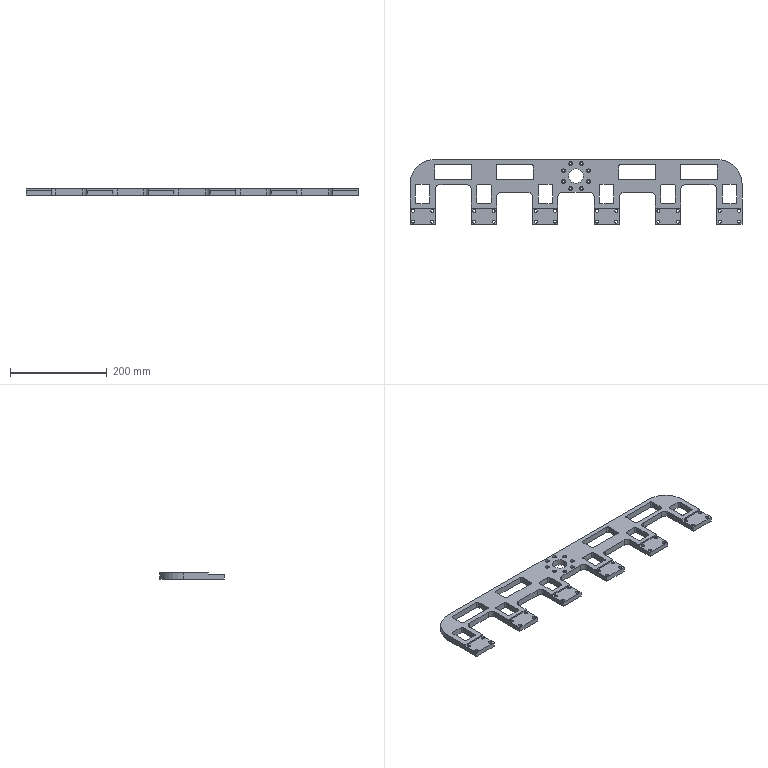NC program | NX | posted with a generic post | part box 687 x 134 x 13 mm
Lines 1 to 122 of 9954:
N10 G17 G21 G94 G90
(FLOOR_WALL_COPY , TOOL : D63)
N12 T01 M6
N14 G54
N16 G17 G0 G90 X-380. Y68.997 S6500 M3
N18 G43 Z30. H1
N20 Z3.
N22 G94 G1 Z0. F1500.
N24 X-377.
N26 X377.
N28 Y40.798
N30 X-377.
N32 Y12.599
N34 X377.
N36 Y-15.601
N38 X-377.
N40 Y-24.911
N42 Y-43.8
N44 X377.
N46 X380.
N48 Z3.
N50 G0 Z30.
N52 M5
(DRILLING_COPY_1 , TOOL : D6A45)
N54 T07 M6
N56 G54
N58 G17 G0 G90 X337.5 Y-39.2 S5000 M3
N60 G43 Z30. H7
N62 G94 G81 G98 Z-1. F250. R3.
N64 Y-61.2
N66 X297.5
N68 Y-39.2
N70 X210.5
N72 Y-61.2
N74 X170.5
N76 Y-39.2
N78 X83.5
N80 Y-61.2
N82 X43.5
N84 Y-39.2
N86 X10.715 Y7.131
N88 X25.869 Y22.285
N90 Y43.715
N92 X10.715 Y58.869
N94 X-10.715
N96 X-25.869 Y43.715
N98 Y22.285
N100 X0. Y33.
N102 X-10.715 Y7.131
N104 X-43.5 Y-39.2
N106 Y-61.2
N108 X-83.5
N110 Y-39.2
N112 X-170.5 Y-61.2
N114 Y-39.2
N116 X-210.5
N118 Y-61.2
N120 X-297.5
N122 Y-39.2
N124 X-337.5
N126 Y-61.2
N128 G80
N130 G0 X-337.5 Y-61.2 Z30.
N132 M5
(DRILLING_COPY_COPY_1 , TOOL : 4.5ZT)
N134 T14 M6
N136 G54
N138 G17 G0 G90 X10.715 Y58.869 S2000 M3
N140 G43 Z30. H14
N142 G94 G83 G98 Z-14.5 F250. Q2. R3.
N144 X-10.715
N146 X-25.869 Y43.715
N148 Y22.285
N150 X-10.715 Y7.131
N152 X10.715
N154 X25.869 Y22.285
N156 Y43.715
N158 G80
N160 G0 X25.869 Y43.715 Z30.
N162 M5
(DRILLING_COPY_COPY_COPY , TOOL : 6.5ZT)
N164 T15 M6
N166 G54
N168 G17 G0 G90 X337.5 Y-39.2 S2000 M3
N170 G43 Z30. H15
N172 G94 G83 G98 Z-14.5 F250. Q2. R3.
N174 Y-61.2
N176 X297.5
N178 Y-39.2
N180 X210.5
N182 Y-61.2
N184 X170.5
N186 Y-39.2
N188 X83.5
N190 Y-61.2
N192 X43.5
N194 Y-39.2
N196 X-43.5
N198 Y-61.2
N200 X-83.5
N202 Y-39.2
N204 X-170.5
N206 Y-61.2
N208 X-210.5
N210 Y-39.2
N212 X-297.5
N214 Y-61.2
N216 X-337.5
N218 Y-39.2
N220 G80
N222 G0 X-337.5 Y-39.2 Z30.
N224 M5